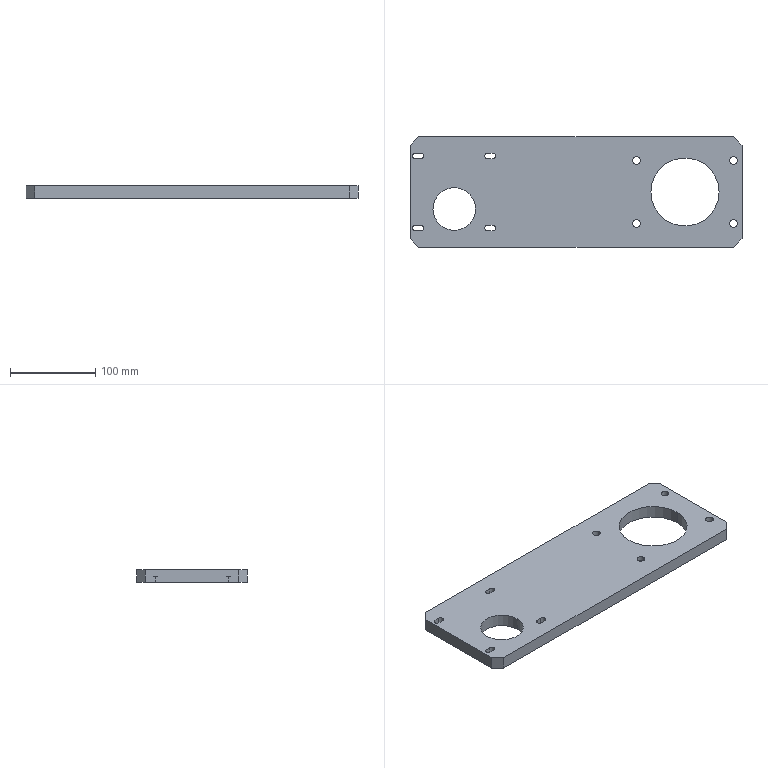Part | SolidWorks | features HoleWzd 2, Chamfer 1, Cut 1, Extrusion 1 | 1 solid | 78 faces | box 390 x 130 x 15 mm | volume 637753 mm3 | cylinder 44 | plane 34 | commonest cylinder face diameters 6.6 x12 11 x12 9 x8 15 x8 50 x2 80 x2